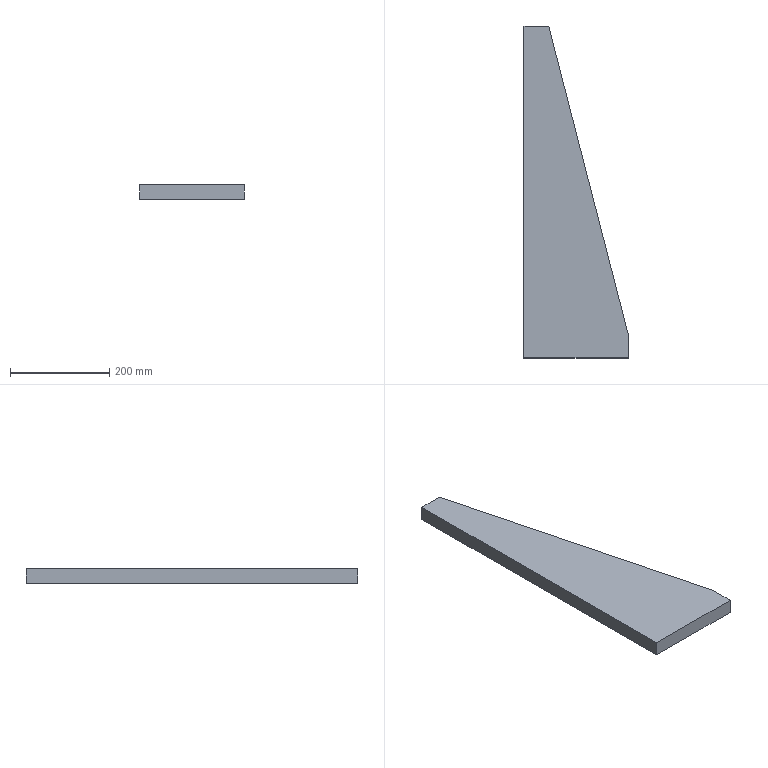Part | SolidWorks | features Extrusion 1 | 1 solid | 7 faces | box 210 x 670 x 30 mm | volume 2733000 mm3 | plane 7
STEP:
#1=CARTESIAN_POINT('',(0.,0.,0.));
#2=VERTEX_POINT('',#1);
#3=CARTESIAN_POINT('',(210.,0.,0.));
#4=VERTEX_POINT('',#3);
#5=CARTESIAN_POINT('',(210.,0.,0.));
#6=DIRECTION('',(1.,0.,0.));
#7=VECTOR('',#6,1000.);
#8=LINE('',#5,#7);
#9=EDGE_CURVE('',#2,#4,#8,.T.);
#10=ORIENTED_EDGE('',*,*,#9,.T.);
#11=CARTESIAN_POINT('',(210.,0.,30.));
#12=VERTEX_POINT('',#11);
#13=CARTESIAN_POINT('',(210.,0.,30.));
#14=DIRECTION('',(0.,0.,-1.));
#15=VECTOR('',#14,1000.);
#16=LINE('',#13,#15);
#17=EDGE_CURVE('',#12,#4,#16,.T.);
#18=ORIENTED_EDGE('',*,*,#17,.F.);
#19=CARTESIAN_POINT('',(0.,0.,30.));
#20=VERTEX_POINT('',#19);
#21=CARTESIAN_POINT('',(210.,0.,30.));
#22=DIRECTION('',(1.,0.,0.));
#23=VECTOR('',#22,1000.);
#24=LINE('',#21,#23);
#25=EDGE_CURVE('',#20,#12,#24,.T.);
#26=ORIENTED_EDGE('',*,*,#25,.F.);
#27=CARTESIAN_POINT('',(0.,0.,30.));
#28=DIRECTION('',(0.,0.,-1.));
#29=VECTOR('',#28,1000.);
#30=LINE('',#27,#29);
#31=EDGE_CURVE('',#20,#2,#30,.T.);
#32=ORIENTED_EDGE('',*,*,#31,.T.);
#33=EDGE_LOOP('',(#10,#18,#26,#32));
#34=FACE_OUTER_BOUND('',#33,.T.);
#35=CARTESIAN_POINT('',(210.,0.,30.));
#36=DIRECTION('',(0.,1.,0.));
#37=DIRECTION('',(-1.,0.,0.));
#38=AXIS2_PLACEMENT_3D('',#35,#36,#37);
#39=PLANE('',#38);
#40=ADVANCED_FACE('',(#34),#39,.F.);
#41=CARTESIAN_POINT('',(210.,50.,0.));
#42=VERTEX_POINT('',#41);
#43=CARTESIAN_POINT('',(210.,50.,0.));
#44=DIRECTION('',(0.,1.,0.));
#45=VECTOR('',#44,1000.);
#46=LINE('',#43,#45);
#47=EDGE_CURVE('',#4,#42,#46,.T.);
#48=ORIENTED_EDGE('',*,*,#47,.T.);
#49=CARTESIAN_POINT('',(210.,50.,30.));
#50=VERTEX_POINT('',#49);
#51=CARTESIAN_POINT('',(210.,50.,30.));
#52=DIRECTION('',(0.,0.,-1.));
#53=VECTOR('',#52,1000.);
#54=LINE('',#51,#53);
#55=EDGE_CURVE('',#50,#42,#54,.T.);
#56=ORIENTED_EDGE('',*,*,#55,.F.);
#57=CARTESIAN_POINT('',(210.,50.,30.));
#58=DIRECTION('',(0.,1.,0.));
#59=VECTOR('',#58,1000.);
#60=LINE('',#57,#59);
#61=EDGE_CURVE('',#12,#50,#60,.T.);
#62=ORIENTED_EDGE('',*,*,#61,.F.);
#63=ORIENTED_EDGE('',*,*,#17,.T.);
#64=EDGE_LOOP('',(#48,#56,#62,#63));
#65=FACE_OUTER_BOUND('',#64,.T.);
#66=CARTESIAN_POINT('',(210.,50.,30.));
#67=DIRECTION('',(-1.,0.,0.));
#68=DIRECTION('',(0.,0.,1.));
#69=AXIS2_PLACEMENT_3D('',#66,#67,#68);
#70=PLANE('',#69);
#71=ADVANCED_FACE('',(#65),#70,.F.);
#72=CARTESIAN_POINT('',(50.,670.,0.));
#73=VERTEX_POINT('',#72);
#74=CARTESIAN_POINT('',(50.,670.,0.));
#75=DIRECTION('',(-0.2499,0.9683,0.));
#76=VECTOR('',#75,1000.);
#77=LINE('',#74,#76);
#78=EDGE_CURVE('',#42,#73,#77,.T.);
#79=ORIENTED_EDGE('',*,*,#78,.T.);
#80=CARTESIAN_POINT('',(50.,670.,30.));
#81=VERTEX_POINT('',#80);
#82=CARTESIAN_POINT('',(50.,670.,30.));
#83=DIRECTION('',(0.,0.,-1.));
#84=VECTOR('',#83,1000.);
#85=LINE('',#82,#84);
#86=EDGE_CURVE('',#81,#73,#85,.T.);
#87=ORIENTED_EDGE('',*,*,#86,.F.);
#88=CARTESIAN_POINT('',(50.,670.,30.));
#89=DIRECTION('',(-0.2499,0.9683,0.));
#90=VECTOR('',#89,1000.);
#91=LINE('',#88,#90);
#92=EDGE_CURVE('',#50,#81,#91,.T.);
#93=ORIENTED_EDGE('',*,*,#92,.F.);
#94=ORIENTED_EDGE('',*,*,#55,.T.);
#95=EDGE_LOOP('',(#79,#87,#93,#94));
#96=FACE_OUTER_BOUND('',#95,.T.);
#97=CARTESIAN_POINT('',(50.,670.,30.));
#98=DIRECTION('',(-0.9683,-0.2499,0.));
#99=DIRECTION('',(0.2499,-0.9683,0.));
#100=AXIS2_PLACEMENT_3D('',#97,#98,#99);
#101=PLANE('',#100);
#102=ADVANCED_FACE('',(#96),#101,.F.);
#103=CARTESIAN_POINT('',(0.,670.,0.));
#104=VERTEX_POINT('',#103);
#105=CARTESIAN_POINT('',(0.,670.,0.));
#106=DIRECTION('',(-1.,0.,0.));
#107=VECTOR('',#106,1000.);
#108=LINE('',#105,#107);
#109=EDGE_CURVE('',#73,#104,#108,.T.);
#110=ORIENTED_EDGE('',*,*,#109,.T.);
#111=CARTESIAN_POINT('',(0.,670.,30.));
#112=VERTEX_POINT('',#111);
#113=CARTESIAN_POINT('',(0.,670.,30.));
#114=DIRECTION('',(0.,0.,-1.));
#115=VECTOR('',#114,1000.);
#116=LINE('',#113,#115);
#117=EDGE_CURVE('',#112,#104,#116,.T.);
#118=ORIENTED_EDGE('',*,*,#117,.F.);
#119=CARTESIAN_POINT('',(0.,670.,30.));
#120=DIRECTION('',(-1.,0.,0.));
#121=VECTOR('',#120,1000.);
#122=LINE('',#119,#121);
#123=EDGE_CURVE('',#81,#112,#122,.T.);
#124=ORIENTED_EDGE('',*,*,#123,.F.);
#125=ORIENTED_EDGE('',*,*,#86,.T.);
#126=EDGE_LOOP('',(#110,#118,#124,#125));
#127=FACE_OUTER_BOUND('',#126,.T.);
#128=CARTESIAN_POINT('',(0.,670.,30.));
#129=DIRECTION('',(0.,-1.,0.));
#130=DIRECTION('',(0.,0.,-1.));
#131=AXIS2_PLACEMENT_3D('',#128,#129,#130);
#132=PLANE('',#131);
#133=ADVANCED_FACE('',(#127),#132,.F.);
#134=CARTESIAN_POINT('',(0.,0.,0.));
#135=DIRECTION('',(0.,-1.,0.));
#136=VECTOR('',#135,1000.);
#137=LINE('',#134,#136);
#138=EDGE_CURVE('',#104,#2,#137,.T.);
#139=ORIENTED_EDGE('',*,*,#138,.T.);
#140=ORIENTED_EDGE('',*,*,#31,.F.);
#141=CARTESIAN_POINT('',(0.,0.,30.));
#142=DIRECTION('',(0.,-1.,0.));
#143=VECTOR('',#142,1000.);
#144=LINE('',#141,#143);
#145=EDGE_CURVE('',#112,#20,#144,.T.);
#146=ORIENTED_EDGE('',*,*,#145,.F.);
#147=ORIENTED_EDGE('',*,*,#117,.T.);
#148=EDGE_LOOP('',(#139,#140,#146,#147));
#149=FACE_OUTER_BOUND('',#148,.T.);
#150=CARTESIAN_POINT('',(0.,0.,30.));
#151=DIRECTION('',(1.,0.,0.));
#152=DIRECTION('',(0.,0.,-1.));
#153=AXIS2_PLACEMENT_3D('',#150,#151,#152);
#154=PLANE('',#153);
#155=ADVANCED_FACE('',(#149),#154,.F.);
#156=ORIENTED_EDGE('',*,*,#25,.T.);
#157=ORIENTED_EDGE('',*,*,#61,.T.);
#158=ORIENTED_EDGE('',*,*,#92,.T.);
#159=ORIENTED_EDGE('',*,*,#123,.T.);
#160=ORIENTED_EDGE('',*,*,#145,.T.);
#161=EDGE_LOOP('',(#156,#157,#158,#159,#160));
#162=FACE_OUTER_BOUND('',#161,.T.);
#163=CARTESIAN_POINT('',(0.,0.,30.));
#164=DIRECTION('',(0.,0.,-1.));
#165=DIRECTION('',(-1.,0.,0.));
#166=AXIS2_PLACEMENT_3D('',#163,#164,#165);
#167=PLANE('',#166);
#168=ADVANCED_FACE('',(#162),#167,.F.);
#169=ORIENTED_EDGE('',*,*,#9,.F.);
#170=ORIENTED_EDGE('',*,*,#138,.F.);
#171=ORIENTED_EDGE('',*,*,#109,.F.);
#172=ORIENTED_EDGE('',*,*,#78,.F.);
#173=ORIENTED_EDGE('',*,*,#47,.F.);
#174=EDGE_LOOP('',(#169,#170,#171,#172,#173));
#175=FACE_OUTER_BOUND('',#174,.T.);
#176=CARTESIAN_POINT('',(0.,0.,0.));
#177=DIRECTION('',(0.,0.,-1.));
#178=DIRECTION('',(-1.,0.,0.));
#179=AXIS2_PLACEMENT_3D('',#176,#177,#178);
#180=PLANE('',#179);
#181=ADVANCED_FACE('',(#175),#180,.T.);
#182=CLOSED_SHELL('',(#40,#71,#102,#133,#155,#168,#181));
#183=MANIFOLD_SOLID_BREP('',#182);
#184=CARTESIAN_POINT('',(0.,0.,0.));
#185=DIRECTION('',(0.,0.,1.));
#186=DIRECTION('',(1.,0.,0.));
#187=AXIS2_PLACEMENT_3D('',#184,#185,#186);
#188=(LENGTH_UNIT()NAMED_UNIT(*)SI_UNIT(.MILLI.,.METRE.));
#189=UNCERTAINTY_MEASURE_WITH_UNIT(LENGTH_MEASURE(0.00001),#188,'','');
#190=(NAMED_UNIT(*)PLANE_ANGLE_UNIT()SI_UNIT($,.RADIAN.));
#191=(NAMED_UNIT(*)SI_UNIT($,.STERADIAN.)SOLID_ANGLE_UNIT());
#192=(GEOMETRIC_REPRESENTATION_CONTEXT(3)GLOBAL_UNCERTAINTY_ASSIGNED_CONTEXT((#189))GLOBAL_UNIT_ASSIGNED_CONTEXT((#188,#190,#191))REPRESENTATION_CONTEXT('',''));
#193=ADVANCED_BREP_SHAPE_REPRESENTATION('',(#183,#187),#192);